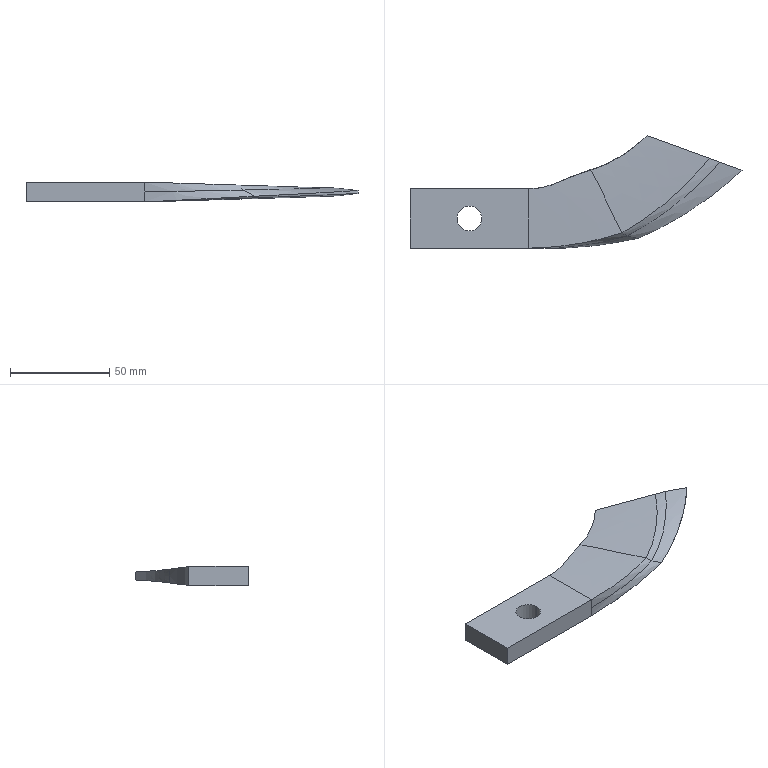Part | SolidWorks | features Blend 1, Extrusion 1 | 1 solid | 22 faces | box 167.64 x 57.038 x 10 mm | volume 39018 mm3 | spline 14 | plane 6 | cylinder 2 | commonest cylinder face diameters 12.5 x2